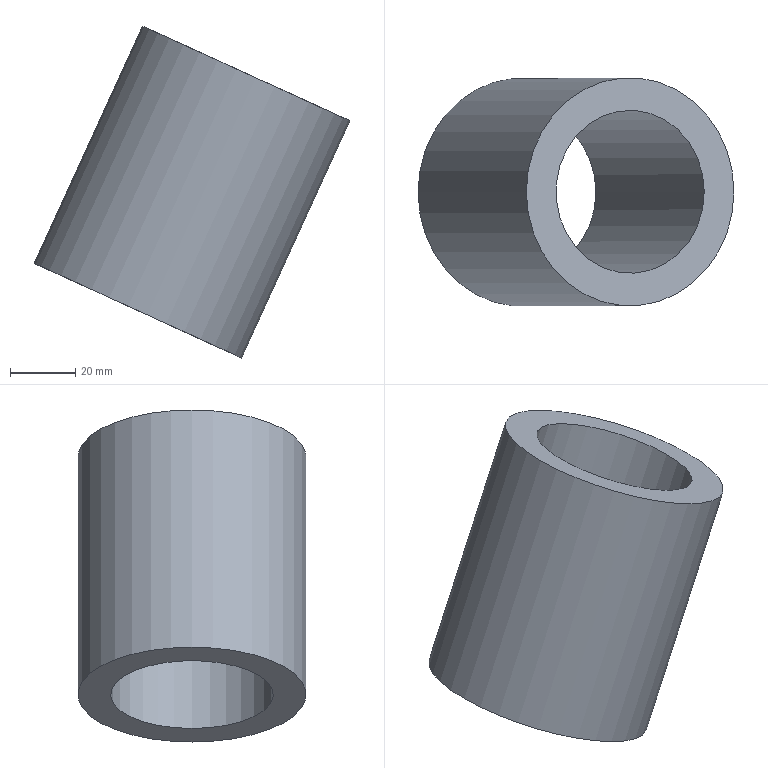Part | STEP file | solid 230 | 1 solid | 4 faces | box 96.9 x 70 x 101.844 mm | volume 150796 mm3 | plane 2 | cylinder 2 | commonest cylinder face diameters 50 x1 70 x1